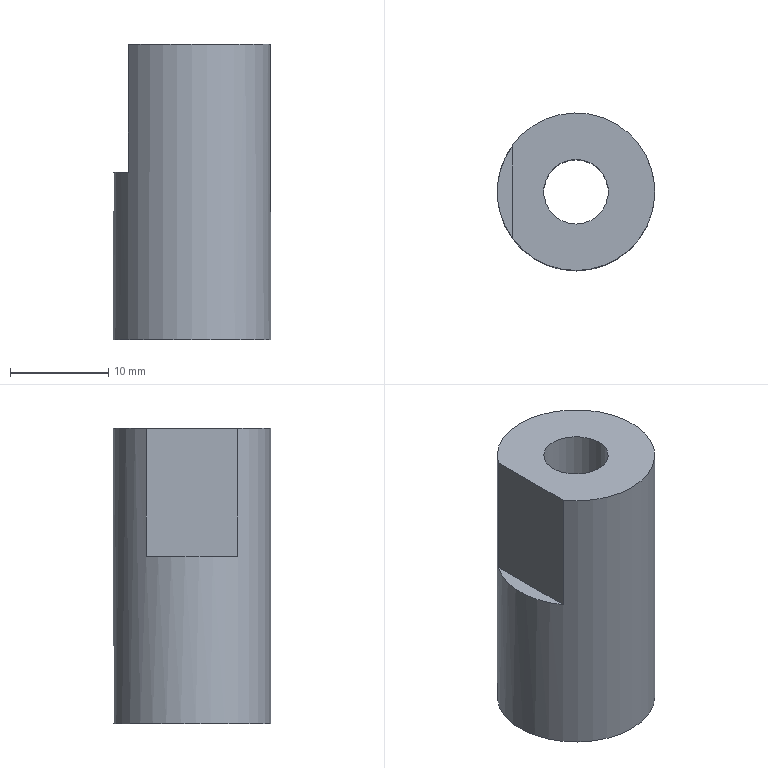Part | STEP file | lll_id66_x_t | 1 solid | 6 faces | box 16 x 16 x 30 mm | volume 4894 mm3 | plane 4 | cylinder 2 | commonest cylinder face diameters 6.56 x1 16 x1
STEP:
#1=CARTESIAN_POINT('',(785.732,24.756,-13.));
#2=VERTEX_POINT('',#1);
#3=CARTESIAN_POINT('',(785.732,34.084,-13.));
#4=VERTEX_POINT('',#3);
#5=CARTESIAN_POINT('',(785.732,29.42,-13.));
#6=DIRECTION('',(0.,1.,0.));
#7=VECTOR('',#6,1.);
#8=LINE('',#5,#7);
#9=EDGE_CURVE('',#2,#4,#8,.T.);
#10=ORIENTED_EDGE('',*,*,#9,.F.);
#11=CARTESIAN_POINT('',(785.732,24.756,0.));
#12=VERTEX_POINT('',#11);
#13=CARTESIAN_POINT('',(785.732,24.756,-13.));
#14=DIRECTION('',(0.,0.,1.));
#15=VECTOR('',#14,1.);
#16=LINE('',#13,#15);
#17=EDGE_CURVE('',#2,#12,#16,.T.);
#18=ORIENTED_EDGE('',*,*,#17,.T.);
#19=CARTESIAN_POINT('',(785.732,34.084,0.));
#20=VERTEX_POINT('',#19);
#21=CARTESIAN_POINT('',(785.732,35.06,0.));
#22=DIRECTION('',(0.,-1.,0.));
#23=VECTOR('',#22,1.);
#24=LINE('',#21,#23);
#25=EDGE_CURVE('',#20,#12,#24,.T.);
#26=ORIENTED_EDGE('',*,*,#25,.F.);
#27=CARTESIAN_POINT('',(785.732,34.084,0.));
#28=DIRECTION('',(0.,0.,-1.));
#29=VECTOR('',#28,1.);
#30=LINE('',#27,#29);
#31=EDGE_CURVE('',#20,#4,#30,.T.);
#32=ORIENTED_EDGE('',*,*,#31,.T.);
#33=EDGE_LOOP('',(#10,#18,#26,#32));
#34=FACE_OUTER_BOUND('',#33,.T.);
#35=CARTESIAN_POINT('',(785.732,35.06,-15.));
#36=DIRECTION('',(1.,0.,0.));
#37=DIRECTION('',(0.,0.,-1.));
#38=AXIS2_PLACEMENT_3D('',#35,#36,#37);
#39=PLANE('',#38);
#40=ADVANCED_FACE('',(#34),#39,.F.);
#41=CARTESIAN_POINT('',(792.232,26.14,-30.));
#42=VERTEX_POINT('',#41);
#43=CARTESIAN_POINT('',(792.232,29.42,-30.));
#44=DIRECTION('',(0.,0.,-1.));
#45=DIRECTION('',(0.,-1.,0.));
#46=AXIS2_PLACEMENT_3D('',#43,#44,#45);
#47=CIRCLE('',#46,3.28);
#48=EDGE_CURVE('',#42,#42,#47,.T.);
#49=ORIENTED_EDGE('',*,*,#48,.F.);
#50=EDGE_LOOP('',(#49));
#51=FACE_BOUND('',#50,.T.);
#52=CARTESIAN_POINT('',(792.232,21.42,-30.));
#53=VERTEX_POINT('',#52);
#54=CARTESIAN_POINT('',(792.232,29.42,-30.));
#55=DIRECTION('',(0.,0.,1.));
#56=DIRECTION('',(0.,-1.,0.));
#57=AXIS2_PLACEMENT_3D('',#54,#55,#56);
#58=CIRCLE('',#57,8.);
#59=EDGE_CURVE('',#53,#53,#58,.T.);
#60=ORIENTED_EDGE('',*,*,#59,.F.);
#61=EDGE_LOOP('',(#60));
#62=FACE_BOUND('',#61,.T.);
#63=CARTESIAN_POINT('',(792.232,29.42,-30.));
#64=DIRECTION('',(0.,0.,-1.));
#65=DIRECTION('',(0.,-1.,0.));
#66=AXIS2_PLACEMENT_3D('',#63,#64,#65);
#67=PLANE('',#66);
#68=ADVANCED_FACE('',(#51,#62),#67,.T.);
#69=CARTESIAN_POINT('',(792.232,32.7,0.));
#70=VERTEX_POINT('',#69);
#71=CARTESIAN_POINT('',(792.232,29.42,0.));
#72=DIRECTION('',(0.,0.,1.));
#73=DIRECTION('',(0.,1.,0.));
#74=AXIS2_PLACEMENT_3D('',#71,#72,#73);
#75=CIRCLE('',#74,3.28);
#76=EDGE_CURVE('',#70,#70,#75,.T.);
#77=ORIENTED_EDGE('',*,*,#76,.F.);
#78=EDGE_LOOP('',(#77));
#79=FACE_BOUND('',#78,.T.);
#80=ORIENTED_EDGE('',*,*,#25,.T.);
#81=CARTESIAN_POINT('',(792.232,29.42,0.));
#82=DIRECTION('',(0.,0.,-1.));
#83=DIRECTION('',(0.,1.,0.));
#84=AXIS2_PLACEMENT_3D('',#81,#82,#83);
#85=CIRCLE('',#84,8.);
#86=EDGE_CURVE('',#20,#12,#85,.T.);
#87=ORIENTED_EDGE('',*,*,#86,.F.);
#88=EDGE_LOOP('',(#80,#87));
#89=FACE_BOUND('',#88,.T.);
#90=CARTESIAN_POINT('',(792.232,29.42,0.));
#91=DIRECTION('',(0.,0.,1.));
#92=DIRECTION('',(0.,1.,0.));
#93=AXIS2_PLACEMENT_3D('',#90,#91,#92);
#94=PLANE('',#93);
#95=ADVANCED_FACE('',(#79,#89),#94,.T.);
#96=ORIENTED_EDGE('',*,*,#59,.T.);
#97=EDGE_LOOP('',(#96));
#98=FACE_BOUND('',#97,.T.);
#99=ORIENTED_EDGE('',*,*,#31,.F.);
#100=ORIENTED_EDGE('',*,*,#86,.T.);
#101=ORIENTED_EDGE('',*,*,#17,.F.);
#102=CARTESIAN_POINT('',(792.232,29.42,-13.));
#103=DIRECTION('',(0.,0.,-1.));
#104=DIRECTION('',(0.,1.,0.));
#105=AXIS2_PLACEMENT_3D('',#102,#103,#104);
#106=CIRCLE('',#105,8.);
#107=EDGE_CURVE('',#2,#4,#106,.T.);
#108=ORIENTED_EDGE('',*,*,#107,.T.);
#109=EDGE_LOOP('',(#99,#100,#101,#108));
#110=FACE_BOUND('',#109,.T.);
#111=CARTESIAN_POINT('',(792.232,29.42,0.));
#112=DIRECTION('',(0.,0.,-1.));
#113=DIRECTION('',(0.,-1.,0.));
#114=AXIS2_PLACEMENT_3D('',#111,#112,#113);
#115=CYLINDRICAL_SURFACE('',#114,8.);
#116=ADVANCED_FACE('',(#98,#110),#115,.T.);
#117=ORIENTED_EDGE('',*,*,#76,.T.);
#118=EDGE_LOOP('',(#117));
#119=FACE_BOUND('',#118,.T.);
#120=ORIENTED_EDGE('',*,*,#48,.T.);
#121=EDGE_LOOP('',(#120));
#122=FACE_BOUND('',#121,.T.);
#123=CARTESIAN_POINT('',(792.232,29.42,52.5));
#124=DIRECTION('',(0.,0.,-1.));
#125=DIRECTION('',(0.,-1.,0.));
#126=AXIS2_PLACEMENT_3D('',#123,#124,#125);
#127=CYLINDRICAL_SURFACE('',#126,3.28);
#128=ADVANCED_FACE('',(#119,#122),#127,.F.);
#129=ORIENTED_EDGE('',*,*,#107,.F.);
#130=ORIENTED_EDGE('',*,*,#9,.T.);
#131=EDGE_LOOP('',(#129,#130));
#132=FACE_OUTER_BOUND('',#131,.T.);
#133=CARTESIAN_POINT('',(792.232,29.42,-13.));
#134=DIRECTION('',(0.,0.,1.));
#135=DIRECTION('',(0.,1.,0.));
#136=AXIS2_PLACEMENT_3D('',#133,#134,#135);
#137=PLANE('',#136);
#138=ADVANCED_FACE('',(#132),#137,.T.);
#139=CLOSED_SHELL('',(#40,#68,#95,#116,#128,#138));
#140=MANIFOLD_SOLID_BREP('',#139);
#141=(LENGTH_UNIT()NAMED_UNIT(*)SI_UNIT(.MILLI.,.METRE.));
#142=UNCERTAINTY_MEASURE_WITH_UNIT(LENGTH_MEASURE(0.00002),#141,'','');
#143=(NAMED_UNIT(*)PLANE_ANGLE_UNIT()SI_UNIT($,.RADIAN.));
#144=PLANE_ANGLE_MEASURE_WITH_UNIT(PLANE_ANGLE_MEASURE(0.01745),#143);
#145=DIMENSIONAL_EXPONENTS(0.,0.,0.,0.,0.,0.,0.);
#146=(CONVERSION_BASED_UNIT('DEGREE',#144)NAMED_UNIT(#145)PLANE_ANGLE_UNIT());
#147=(NAMED_UNIT(*)SI_UNIT($,.STERADIAN.)SOLID_ANGLE_UNIT());
#148=(GEOMETRIC_REPRESENTATION_CONTEXT(3)GLOBAL_UNCERTAINTY_ASSIGNED_CONTEXT((#142))GLOBAL_UNIT_ASSIGNED_CONTEXT((#141,#146,#147))REPRESENTATION_CONTEXT('',''));
#149=ADVANCED_BREP_SHAPE_REPRESENTATION('',(#140),#148);